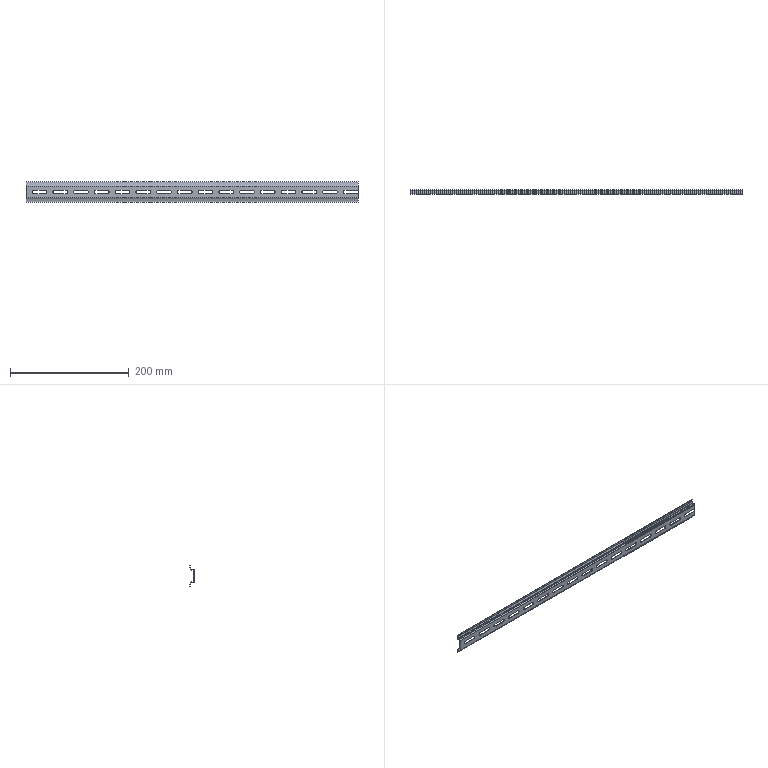Part | SolidWorks | features BaseBody 1 | 1 solid | 100 faces | box 560 x 7.5 x 35.04 mm | volume 23497 mm3 | plane 51 | cylinder 49 | commonest cylinder face diameters 5.352 x33 1.473 x8 3.473 x8